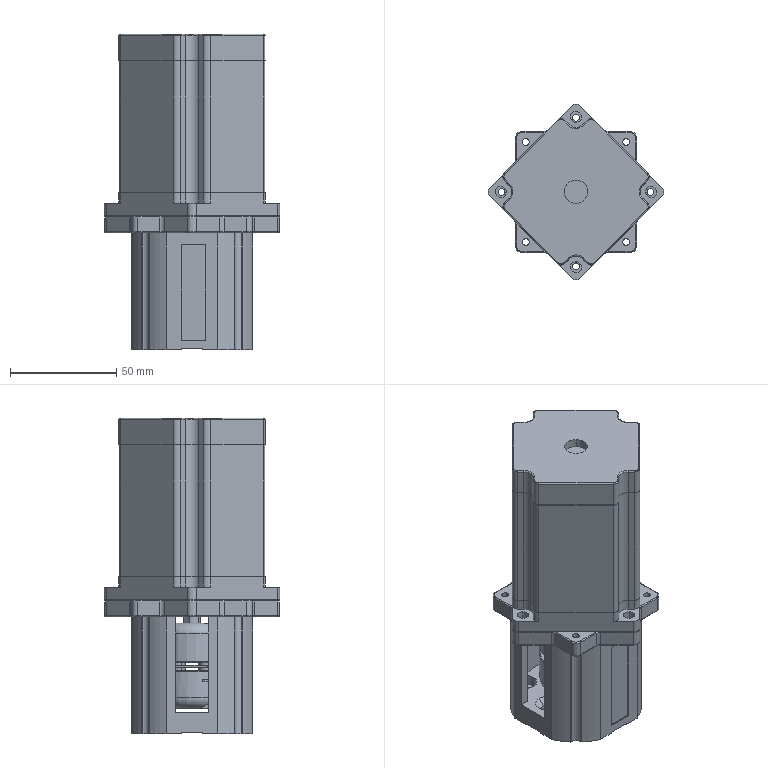Part | STEP file | Copy of 60 motor assembly (universal motor base)^K50A-1H20-S(formula driven)-L300-motor left- | 3 solids | 591 faces | box 82.65 x 82.65 x 148.5 mm | volume 366455 mm3 | cylinder 283 | plane 202 | torus 49 | cone 45 | spline 12 | commonest cylinder face diameters 1 x52 7 x32 6 x26 5 x24 8 x23 3.3 x21